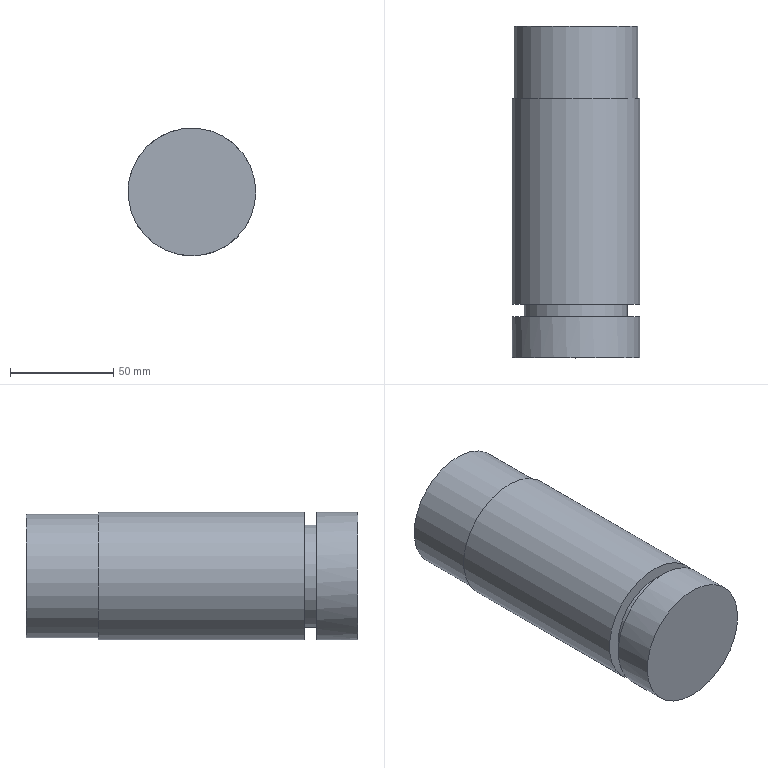Part | NX | features solid 2 | 1 solid | 9 faces | box 62 x 161 x 62 mm | volume 473030 mm3 | plane 5 | cylinder 4 | commonest cylinder face diameters 62 x2 50 x1 60 x1
STEP:
#1=CARTESIAN_POINT('',(-590.,-816.,134.));
#2=VERTEX_POINT('',#1);
#3=CARTESIAN_POINT('',(-590.,-816.,165.));
#4=DIRECTION('',(0.,-1.,0.));
#5=DIRECTION('',(0.,0.,-1.));
#6=AXIS2_PLACEMENT_3D('',#3,#4,#5);
#7=CIRCLE('',#6,31.);
#8=EDGE_CURVE('',#2,#2,#7,.T.);
#9=ORIENTED_EDGE('',*,*,#8,.T.);
#10=EDGE_LOOP('',(#9));
#11=FACE_BOUND('',#10,.T.);
#12=CARTESIAN_POINT('',(-590.,-816.,165.));
#13=DIRECTION('',(0.,-1.,0.));
#14=DIRECTION('',(0.,0.,-1.));
#15=AXIS2_PLACEMENT_3D('',#12,#13,#14);
#16=PLANE('',#15);
#17=ADVANCED_FACE('',(#11),#16,.T.);
#18=CARTESIAN_POINT('',(-559.,-790.,165.));
#19=VERTEX_POINT('',#18);
#20=CARTESIAN_POINT('',(-590.,-790.,165.));
#21=DIRECTION('',(0.,-1.,0.));
#22=DIRECTION('',(1.,0.,0.));
#23=AXIS2_PLACEMENT_3D('',#20,#21,#22);
#24=CIRCLE('',#23,31.);
#25=EDGE_CURVE('',#19,#19,#24,.T.);
#26=ORIENTED_EDGE('',*,*,#25,.T.);
#27=EDGE_LOOP('',(#26));
#28=FACE_BOUND('',#27,.T.);
#29=CARTESIAN_POINT('',(-565.,-790.,165.));
#30=VERTEX_POINT('',#29);
#31=CARTESIAN_POINT('',(-590.,-790.,165.));
#32=DIRECTION('',(0.,-1.,0.));
#33=DIRECTION('',(1.,0.,0.));
#34=AXIS2_PLACEMENT_3D('',#31,#32,#33);
#35=CIRCLE('',#34,25.);
#36=EDGE_CURVE('',#30,#30,#35,.T.);
#37=ORIENTED_EDGE('',*,*,#36,.F.);
#38=EDGE_LOOP('',(#37));
#39=FACE_BOUND('',#38,.T.);
#40=CARTESIAN_POINT('',(-590.,-790.,165.));
#41=DIRECTION('',(0.,-1.,0.));
#42=DIRECTION('',(0.,0.,-1.));
#43=AXIS2_PLACEMENT_3D('',#40,#41,#42);
#44=PLANE('',#43);
#45=ADVANCED_FACE('',(#28,#39),#44,.T.);
#46=ORIENTED_EDGE('',*,*,#25,.F.);
#47=EDGE_LOOP('',(#46));
#48=FACE_BOUND('',#47,.T.);
#49=CARTESIAN_POINT('',(-559.,-690.,165.));
#50=VERTEX_POINT('',#49);
#51=CARTESIAN_POINT('',(-590.,-690.,165.));
#52=DIRECTION('',(0.,-1.,0.));
#53=DIRECTION('',(1.,0.,0.));
#54=AXIS2_PLACEMENT_3D('',#51,#52,#53);
#55=CIRCLE('',#54,31.);
#56=EDGE_CURVE('',#50,#50,#55,.T.);
#57=ORIENTED_EDGE('',*,*,#56,.T.);
#58=EDGE_LOOP('',(#57));
#59=FACE_BOUND('',#58,.T.);
#60=CARTESIAN_POINT('',(-590.,-790.,165.));
#61=DIRECTION('',(0.,1.,0.));
#62=DIRECTION('',(0.,0.,1.));
#63=AXIS2_PLACEMENT_3D('',#60,#61,#62);
#64=CYLINDRICAL_SURFACE('',#63,31.);
#65=ADVANCED_FACE('',(#48,#59),#64,.T.);
#66=CARTESIAN_POINT('',(-560.,-690.,165.));
#67=VERTEX_POINT('',#66);
#68=CARTESIAN_POINT('',(-590.,-690.,165.));
#69=DIRECTION('',(0.,-1.,0.));
#70=DIRECTION('',(1.,0.,0.));
#71=AXIS2_PLACEMENT_3D('',#68,#69,#70);
#72=CIRCLE('',#71,30.);
#73=EDGE_CURVE('',#67,#67,#72,.T.);
#74=ORIENTED_EDGE('',*,*,#73,.T.);
#75=EDGE_LOOP('',(#74));
#76=FACE_BOUND('',#75,.T.);
#77=ORIENTED_EDGE('',*,*,#56,.F.);
#78=EDGE_LOOP('',(#77));
#79=FACE_BOUND('',#78,.T.);
#80=CARTESIAN_POINT('',(-590.,-690.,165.));
#81=DIRECTION('',(0.,-1.,0.));
#82=DIRECTION('',(0.,0.,-1.));
#83=AXIS2_PLACEMENT_3D('',#80,#81,#82);
#84=PLANE('',#83);
#85=ADVANCED_FACE('',(#76,#79),#84,.F.);
#86=CARTESIAN_POINT('',(-560.,-655.,165.));
#87=VERTEX_POINT('',#86);
#88=CARTESIAN_POINT('',(-590.,-655.,165.));
#89=DIRECTION('',(0.,-1.,0.));
#90=DIRECTION('',(1.,0.,0.));
#91=AXIS2_PLACEMENT_3D('',#88,#89,#90);
#92=CIRCLE('',#91,30.);
#93=EDGE_CURVE('',#87,#87,#92,.T.);
#94=ORIENTED_EDGE('',*,*,#93,.T.);
#95=EDGE_LOOP('',(#94));
#96=FACE_BOUND('',#95,.T.);
#97=ORIENTED_EDGE('',*,*,#73,.F.);
#98=EDGE_LOOP('',(#97));
#99=FACE_BOUND('',#98,.T.);
#100=CARTESIAN_POINT('',(-590.,-655.,165.));
#101=DIRECTION('',(0.,-1.,0.));
#102=DIRECTION('',(0.,0.,-1.));
#103=AXIS2_PLACEMENT_3D('',#100,#101,#102);
#104=CYLINDRICAL_SURFACE('',#103,30.);
#105=ADVANCED_FACE('',(#96,#99),#104,.T.);
#106=ORIENTED_EDGE('',*,*,#93,.F.);
#107=EDGE_LOOP('',(#106));
#108=FACE_BOUND('',#107,.T.);
#109=CARTESIAN_POINT('',(-590.,-655.,165.));
#110=DIRECTION('',(0.,-1.,0.));
#111=DIRECTION('',(0.,0.,-1.));
#112=AXIS2_PLACEMENT_3D('',#109,#110,#111);
#113=PLANE('',#112);
#114=ADVANCED_FACE('',(#108),#113,.F.);
#115=CARTESIAN_POINT('',(-565.,-796.,165.));
#116=VERTEX_POINT('',#115);
#117=CARTESIAN_POINT('',(-590.,-796.,165.));
#118=DIRECTION('',(0.,-1.,0.));
#119=DIRECTION('',(1.,0.,0.));
#120=AXIS2_PLACEMENT_3D('',#117,#118,#119);
#121=CIRCLE('',#120,25.);
#122=EDGE_CURVE('',#116,#116,#121,.T.);
#123=ORIENTED_EDGE('',*,*,#122,.F.);
#124=EDGE_LOOP('',(#123));
#125=FACE_BOUND('',#124,.T.);
#126=ORIENTED_EDGE('',*,*,#36,.T.);
#127=EDGE_LOOP('',(#126));
#128=FACE_BOUND('',#127,.T.);
#129=CARTESIAN_POINT('',(-590.,-796.,165.));
#130=DIRECTION('',(0.,1.,0.));
#131=DIRECTION('',(0.,0.,1.));
#132=AXIS2_PLACEMENT_3D('',#129,#130,#131);
#133=CYLINDRICAL_SURFACE('',#132,25.);
#134=ADVANCED_FACE('',(#125,#128),#133,.T.);
#135=CARTESIAN_POINT('',(-559.,-796.,165.));
#136=VERTEX_POINT('',#135);
#137=CARTESIAN_POINT('',(-590.,-796.,165.));
#138=DIRECTION('',(0.,-1.,0.));
#139=DIRECTION('',(1.,0.,0.));
#140=AXIS2_PLACEMENT_3D('',#137,#138,#139);
#141=CIRCLE('',#140,31.);
#142=EDGE_CURVE('',#136,#136,#141,.T.);
#143=ORIENTED_EDGE('',*,*,#142,.F.);
#144=EDGE_LOOP('',(#143));
#145=FACE_BOUND('',#144,.T.);
#146=ORIENTED_EDGE('',*,*,#122,.T.);
#147=EDGE_LOOP('',(#146));
#148=FACE_BOUND('',#147,.T.);
#149=CARTESIAN_POINT('',(-590.,-796.,165.));
#150=DIRECTION('',(0.,-1.,0.));
#151=DIRECTION('',(0.,0.,-1.));
#152=AXIS2_PLACEMENT_3D('',#149,#150,#151);
#153=PLANE('',#152);
#154=ADVANCED_FACE('',(#145,#148),#153,.F.);
#155=ORIENTED_EDGE('',*,*,#8,.F.);
#156=EDGE_LOOP('',(#155));
#157=FACE_BOUND('',#156,.T.);
#158=ORIENTED_EDGE('',*,*,#142,.T.);
#159=EDGE_LOOP('',(#158));
#160=FACE_BOUND('',#159,.T.);
#161=CARTESIAN_POINT('',(-590.,-810.,165.));
#162=DIRECTION('',(0.,1.,0.));
#163=DIRECTION('',(0.,0.,1.));
#164=AXIS2_PLACEMENT_3D('',#161,#162,#163);
#165=CYLINDRICAL_SURFACE('',#164,31.);
#166=ADVANCED_FACE('',(#157,#160),#165,.T.);
#167=CLOSED_SHELL('',(#17,#45,#65,#85,#105,#114,#134,#154,#166));
#168=MANIFOLD_SOLID_BREP('',#167);
#169=(LENGTH_UNIT()NAMED_UNIT(*)SI_UNIT(.MILLI.,.METRE.));
#170=UNCERTAINTY_MEASURE_WITH_UNIT(LENGTH_MEASURE(0.00001),#169,'','');
#171=(NAMED_UNIT(*)PLANE_ANGLE_UNIT()SI_UNIT($,.RADIAN.));
#172=(NAMED_UNIT(*)SI_UNIT($,.STERADIAN.)SOLID_ANGLE_UNIT());
#173=(GEOMETRIC_REPRESENTATION_CONTEXT(3)GLOBAL_UNCERTAINTY_ASSIGNED_CONTEXT((#170))GLOBAL_UNIT_ASSIGNED_CONTEXT((#169,#171,#172))REPRESENTATION_CONTEXT('',''));
#174=ADVANCED_BREP_SHAPE_REPRESENTATION('',(#168),#173);